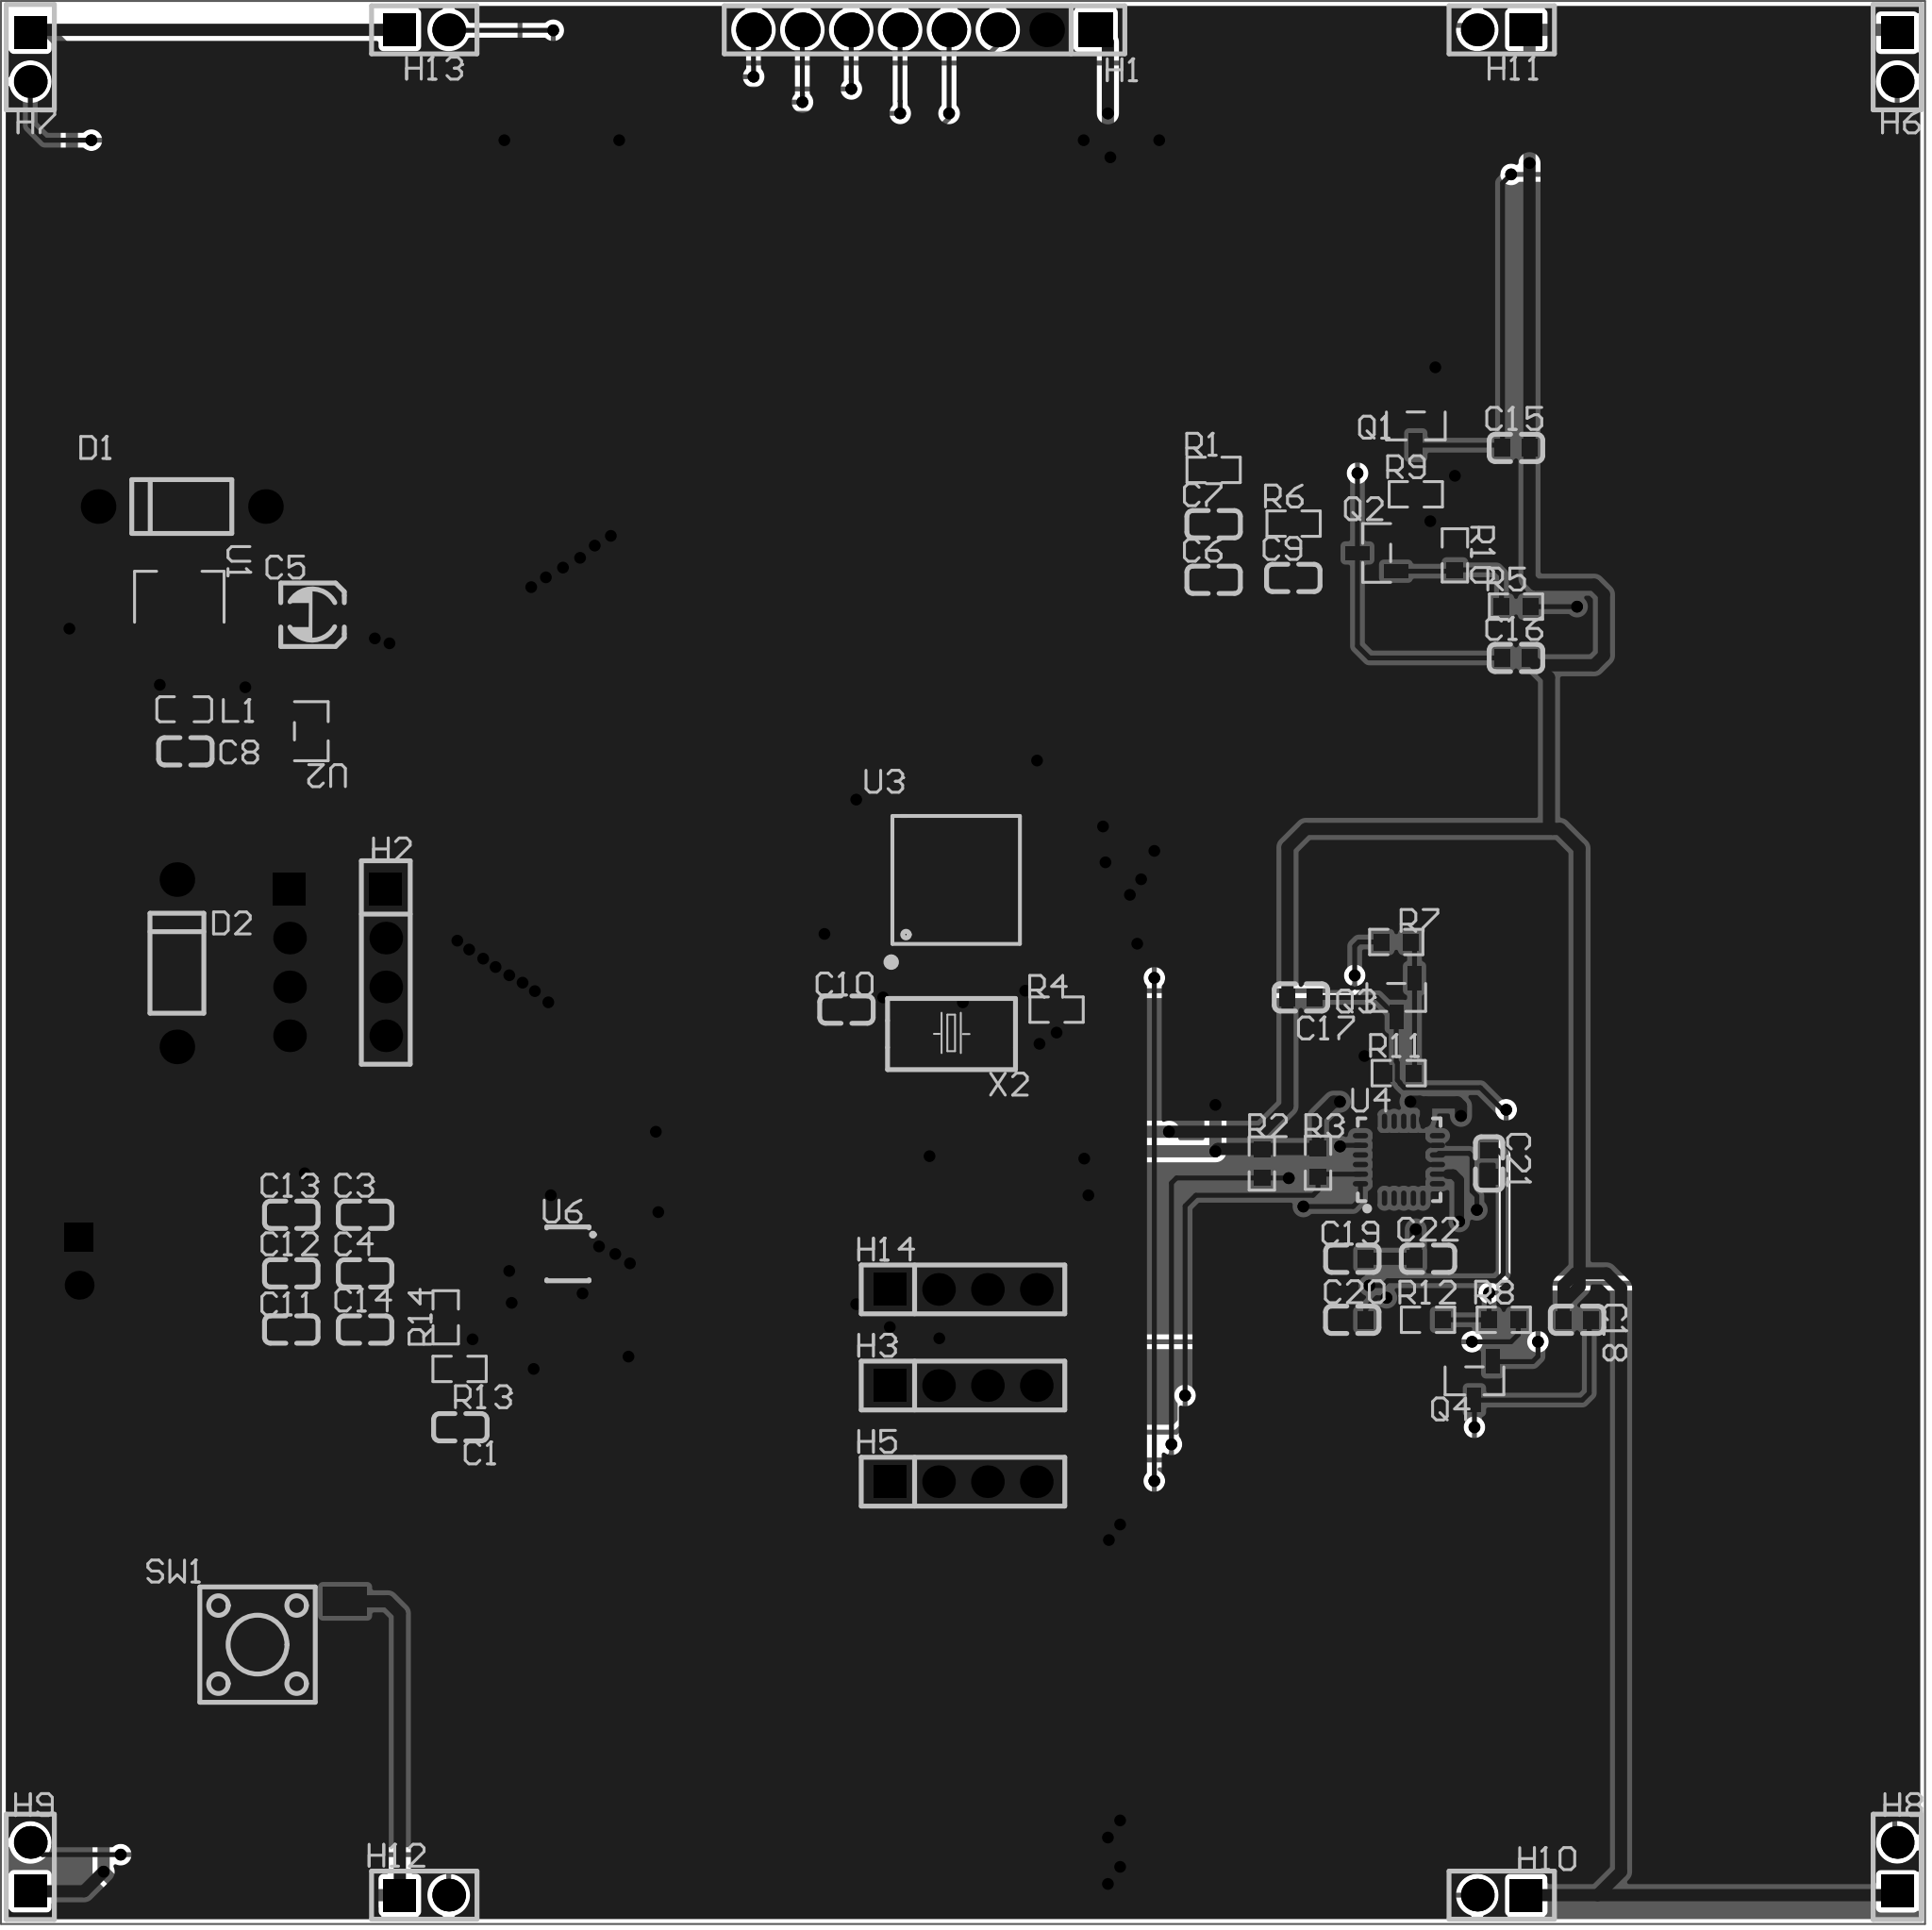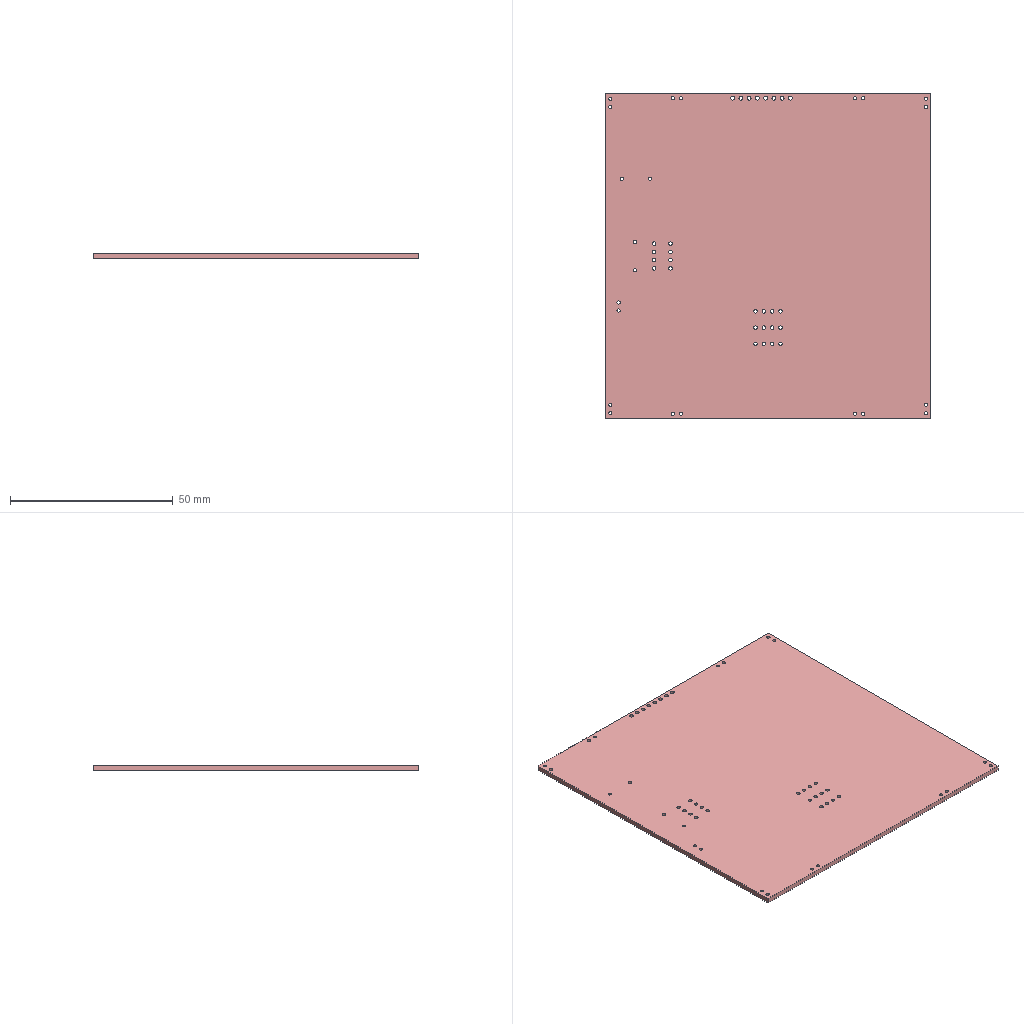Circuit board layout | Altium Designer | box 100 x 100 x 1.6 mm
Layer stack:
# Altium Designer layer stack of  (unit mm; dielectric type: 0 none, 1 core, 2 prepreg, 3 surface material)
index,name,kind,layer,copper_thickness_mm,dielectric_type,dielectric_thickness_mm,dielectric_material,dielectric_constant
0,Top Paste Mask Layer,other,,,,,,
1,Top Silkscreen Layer,other,,,,,,
2,Top Solder Mask Layer,dielectric,,,3,0.01,,3.3
3,Top Layer,copper,Top Layer,0.035,,,,
4,Dielectric1,dielectric,,,3,1.51,FR4,4.5
5,Bottom Layer,copper,Bottom Layer,0.035,,,,
6,Bottom Solder Mask Layer,dielectric,,,3,0.01,,3.3
7,Bottom Silkscreen Layer,other,,,,,,
8,Bottom Paste Mask Layer,other,,,,,,
# drill layer pairs: low layer,high layer
drill_pair,Top Layer,Bottom Layer
Part placement:
Designator,Comment,Layer,Footprint,Center-X(mm),Center-Y(mm),Rotation
C3,20pF,TopLayer,C0603,95.123,113.081,0
C4,20pF,TopLayer,C0603,95.123,110.033,0
C5,0.1uF,TopLayer,C_Ele_SMD_3x5.4mm,92.394,144.279,0
C6,0.1uF,TopLayer,C0603,139.226,146.101,0
C7,0.1uF,TopLayer,C0603,139.226,148.992,0
C8,0.1uF,TopLayer,C0603,85.783,137.18,180
C9,22pF,TopLayer,C0603,143.366,146.197,0
C10,0.1uF,TopLayer,C0603,120.142,123.749,0
C11,0.1uF,TopLayer,C0603,91.287,107.112,0
C12,0.1uF,TopLayer,C0603,91.287,110.037,0
C13,0.1uF,TopLayer,C0603,91.287,113.081,0
C14,0.1uF,TopLayer,C0603,95.123,107.112,0
C15,0.1uF,TopLayer,C0603,154.94,152.959,0
C16,0.1uF,TopLayer,C0603,154.94,142.037,0
C17,0.1uF,TopLayer,C0603,143.764,124.384,180
C18,0.1uF,TopLayer,C0603,158.115,107.62,180
C19,10nF,TopLayer,C0603,146.436,110.794,0
C20,0.1uF,TopLayer,C0603,146.431,107.62,0
C21,2.2nF,TopLayer,C0603,153.543,115.748,270
C22,0.1uF,TopLayer,C0603,150.368,110.795,0
CN1,HX-XH2.54-2PZZ,BottomLayer,CONN-TH_2P-P2.50_HX-2.54MM-2P-ZZ-MS,80.264,110.668,270
D1,,TopLayer,DO_1N4007,85.598,149.911,0
D2,,TopLayer,DO_1N4007,85.344,126.162,270
H1,,TopLayer,HDR-TH_8P-P2.54-V-F-1,124.2,174.7,180
H2,,TopLayer,HDR-TH_4P-P2.54-V-F,96.2,126.2,270
H3,,TopLayer,HDR-TH_4P-P2.54-V-F,126.2,104.2,0
H4,,BottomLayer,HDR-TH_4P-P2.54-V-F,91.2,126.2,270
H5,,TopLayer,HDR-TH_4P-P2.54-V-F,126.2,99.2,0
H6,,TopLayer,HDR-TH_2P-P2.54-V-F,174.752,173.279,270
H7,,TopLayer,HDR-TH_2P-P2.54-V-F,77.724,173.279,270
H8,,TopLayer,HDR-TH_2P-P2.54-V-F,174.752,79.172,90
H9,,TopLayer,HDR-TH_2P-P2.54-V-F,77.724,79.172,90
H10,,TopLayer,HDR-TH_2P-P2.54-V-F,154.2,77.7,180
H11,,TopLayer,HDR-TH_2P-P2.54-V-F,154.2,174.7,180
H12,,TopLayer,HDR-TH_2P-P2.54-V-F,98.2,77.7,0
H13,,TopLayer,HDR-TH_2P-P2.54-V-F,98.2,174.7,0
L1,47uH,TopLayer,L0603,85.725,139.37,0
Q1,,TopLayer,SOT-23-3_L2.9-W1.3-P1.90-LS2.4-BR,149.733,154.102,90
Q2,,TopLayer,SOT-23-3_L2.9-W1.3-P1.90-LS2.4-BR,147.701,147.498,0
Q3,,TopLayer,SOT-23-3_L2.9-W1.3-P1.90-LS2.4-BR,148.717,124.384,90
Q4,,TopLayer,SOT-23-3_L2.9-W1.3-P1.90-LS2.4-BR,152.781,104.445,90
R1,100R,TopLayer,R0603,139.226,151.816,180
R2,4.7K,TopLayer,R0603,141.732,115.748,90
R3,4.7K,TopLayer,R0603,144.651,115.789,90
R4,100R,TopLayer,R0603,131.064,123.749,0
R5,100R,TopLayer,R0603,154.94,144.704,0
R6,100R,TopLayer,R0603,143.383,149.022,0
R7,100R,TopLayer,R0603,148.718,127.266,180
R8,100R,TopLayer,R0603,154.305,107.62,0
R9,10K,TopLayer,R0603,149.733,150.546,0
R10,10K,TopLayer,R0603,151.765,147.371,270
R11,10K,TopLayer,R0603,148.844,120.447,0
R12,10K,TopLayer,R0603,150.368,107.62,0
U1,78L05,TopLayer,SOT-89-3_L4.5-W2.5-P1.50-LS4.2-BR,85.469,144.4,270
U2,XC6206P332MR-G,TopLayer,SOT-23-3_L2.9-W1.6-P1.90-LS2.8-BR,92.329,138.227,180
U3,STM32G474CBT6,TopLayer,LQFP-48_L7.0-W7.0-P0.50-LS9.0-BL,125.857,130.48,0
U4,MPU-6050,TopLayer,QFN-24_L4.0-W4.0-P0.50-BL-EP2.7,148.857,115.943,0
X2,8MHz,TopLayer,CRYSTAL-SMD_L5.0-W3.2,125.603,122.479,180
C1,100nF,TopLayer,C0603,100.076,102.032,0
H14,,TopLayer,HDR-TH_4P-P2.54-V-F,126.2,109.2,0
R13,4.7K,TopLayer,R0603,100.035,105.066,180
R14,4.7K,TopLayer,R0603,99.314,107.747,90
U6,BMP280,TopLayer,LGA-8_L2.5-W2.0-P0.65_AMP6127,105.664,111.049,0
SW1,KH-6X6X5H-STM,TopLayer,SW-SMD_4P-L6.0-W6.0-P4.50-LS9.0_H5.0,89.535,90.729,0
Pad and via stacks:
# Altium Designer via and pad stacks of  (unit mm). Each distinct definition once, with the count of objects using it.
# via: kind,start_layer,end_layer,hole_mm,diameter_mm,mode(0 simple;1 top-mid-bottom;2 full stack),diameter_per_layer,count,example_net
# pad: kind,layer,hole_mm,hole_type(0 round;1 square;2 slot),plating,top_size,top_shape(1 round;2 rect;3 octagon;9 rounded rect),mid_size,bottom_size,mode,footprint,size_per_layer,count,example
pad,Top Layer,0,0,plated,0.8x0.9,2,0.8x0.9,0.8x0.9,0,C0603,,40,C3.2
pad,Top Layer,0,0,plated,1.999x0.8001,2,1.999x0.8001,1.999x0.8001,0,C_Ele_SMD_3x5.4mm,,2,C5.1
pad,Top Layer,0,0,plated,0.8x0.864,2,0.8x0.864,0.8x0.864,0,L0603,,2,L1.1
pad,Top Layer,0,0,plated,1.25x0.7,2,1.25x0.7,1.25x0.7,0,SOT-23-3_L2.9-W1.3-P1.90-LS2.4-BR,,12,Q1.1
pad,Top Layer,0,0,plated,0.8065x0.864,2,0.8065x0.864,0.8065x0.864,0,R0603,,28,R1.2
pad,Top Layer,0,0,plated,1.575x0.672,2,1.575x0.672,1.575x0.672,0,SOT-89-3_L4.5-W2.5-P1.50-LS4.2-BR,,2,U1.1
pad,Top Layer,0,0,plated,0.95x0.95,1,0.95x0.95,0.95x0.95,0,SOT-89-3_L4.5-W2.5-P1.50-LS4.2-BR,,1,U1.2
pad,Top Layer,0,0,plated,1.07x0.6,2,1.07x0.6,1.07x0.6,0,SOT-23-3_L2.9-W1.6-P1.90-LS2.8-BR,,3,U2.1
pad,Top Layer,0,0,plated,0.27x1.5,1,0.27x1.5,0.27x1.5,0,LQFP-48_L7.0-W7.0-P0.50-LS9.0-BL,,24,U3.1
pad,Top Layer,0,0,plated,1.5x0.27,1,1.5x0.27,1.5x0.27,0,LQFP-48_L7.0-W7.0-P0.50-LS9.0-BL,,24,U3.13
pad,Top Layer,0,0,plated,0.28x0.8,1,0.28x0.8,0.28x0.8,0,QFN-24_L4.0-W4.0-P0.50-BL-EP2.7,,12,U4.1
pad,Top Layer,0,0,plated,0.8x0.28,1,0.8x0.28,0.8x0.28,0,QFN-24_L4.0-W4.0-P0.50-BL-EP2.7,,12,U4.7
pad,Top Layer,0,0,plated,2.7x2.7,2,2.7x2.7,2.7x2.7,0,QFN-24_L4.0-W4.0-P0.50-BL-EP2.7,,1,U4.25
pad,Top Layer,0,0,plated,1.9x2.4,2,1.9x2.4,1.9x2.4,0,CRYSTAL-SMD_L5.0-W3.2,,2,X2.2
pad,Top Layer,0,0,plated,0.6x0.4,2,0.6x0.4,0.6x0.4,0,LGA-8_L2.5-W2.0-P0.65_AMP6127,,8,U6.5
pad,Top Layer,0,0,plated,2.3x1.5,2,2.3x1.5,2.3x1.5,0,SW-SMD_4P-L6.0-W6.0-P4.50-LS9.0_H5.0,,4,SW1.1
pad,Multi-Layer,1,0,plated,1.5x1.5,2,1.5x1.5,1.5x1.5,0,CONN-TH_2P-P2.50_HX-2.54MM-2P-ZZ-MS,,1,CN1.1
pad,Multi-Layer,1,0,plated,1.5x1.5,1,1.5x1.5,1.5x1.5,0,CONN-TH_2P-P2.50_HX-2.54MM-2P-ZZ-MS,,1,CN1.2
pad,Multi-Layer,1,0,plated,1.8x1.8,1,1.8x1.8,1.8x1.8,0,DO_1N4007,,4,D1.1
pad,Multi-Layer,1.2,0,plated,1.8x1.8,2,1.8x1.8,1.8x1.8,0,HDR-TH_8P-P2.54-V-F-1,,1,H1.1
pad,Multi-Layer,1.2,0,plated,1.8x1.8,1,1.8x1.8,1.8x1.8,0,HDR-TH_8P-P2.54-V-F-1,,7,H1.2
pad,Multi-Layer,1.1,0,plated,1.7x1.7,2,1.7x1.7,1.7x1.7,0,HDR-TH_4P-P2.54-V-F,,5,H2.1
pad,Multi-Layer,1.1,0,plated,1.7x1.7,1,1.7x1.7,1.7x1.7,0,HDR-TH_4P-P2.54-V-F,,15,H2.2
pad,Multi-Layer,1,0,plated,1.7x1.7,2,1.7x1.7,1.7x1.7,0,HDR-TH_2P-P2.54-V-F,,8,H6.1
pad,Multi-Layer,1,0,plated,1.7x1.7,1,1.7x1.7,1.7x1.7,0,HDR-TH_2P-P2.54-V-F,,8,H6.2
via,Top Layer,Bottom Layer,0.3048,0.61,0,,105,SWCLK
Copper pours:
name,layer,net,type(0 solid;1 hatched;2 none)
Top Layer-GND,Top Layer,GND,0
Bottom Layer-GND,Bottom Layer,GND,0
Design rules, without the lines most boards share:
# Altium Designer design rules of  (exported by Altium Designer, unit mm)
# columns: name | kind | enabled | priority | scope1 | scope2 | descriptor | typed fields (field=value)
copperRegion_Top Layer | 20 | enabled | 1 | (InNet('GND')) And OnLayer('Top Layer') | All | Polygon Connect Rule(Direct Connect )(Conductor Width=10mil) (Relief Angle=90 Angle) (Entries=4) (Air Gap Width=10mil) ((InNet('GND')) And OnLayer('Top Layer')),(All) | connect_style(0=relief,1=direct,2=none)=1 relief_conductor_width=0.254 relief_entries=4
copperRegion_Bottom Layer | 20 | enabled | 2 | (InNet('GND')) And OnLayer('Bottom Layer') | All | Polygon Connect Rule(Direct Connect )(Conductor Width=10mil) (Relief Angle=90 Angle) (Entries=4) (Air Gap Width=10mil) ((InNet('GND')) And OnLayer('Bottom Layer')),(All) | connect_style(0=relief,1=direct,2=none)=1 relief_conductor_width=0.254 relief_entries=4
copperRegion | 20 | enabled | 3 | (InNet('GND')) | All | Polygon Connect Rule(Direct Connect )(Conductor Width=10mil) (Relief Angle=90 Angle) (Entries=4) (Air Gap Width=10mil) ((InNet('GND'))),(All) | connect_style(0=relief,1=direct,2=none)=1 relief_conductor_width=0.254 relief_entries=4